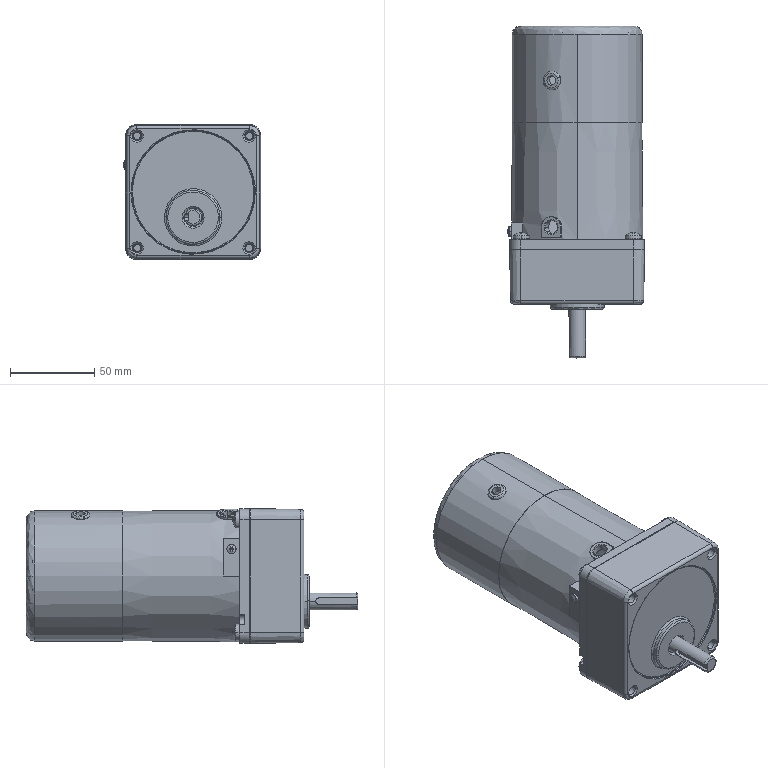Part | SolidWorks | 11 solids | 1373 faces | box 81.315 x 196.821 x 80 mm | volume 357244 mm3 | cone 688 | cylinder 395 | plane 200 | spline 90 | commonest cylinder face diameters 5 x192 4 x94 3 x32 5.5 x8 8 x8 9.5 x8